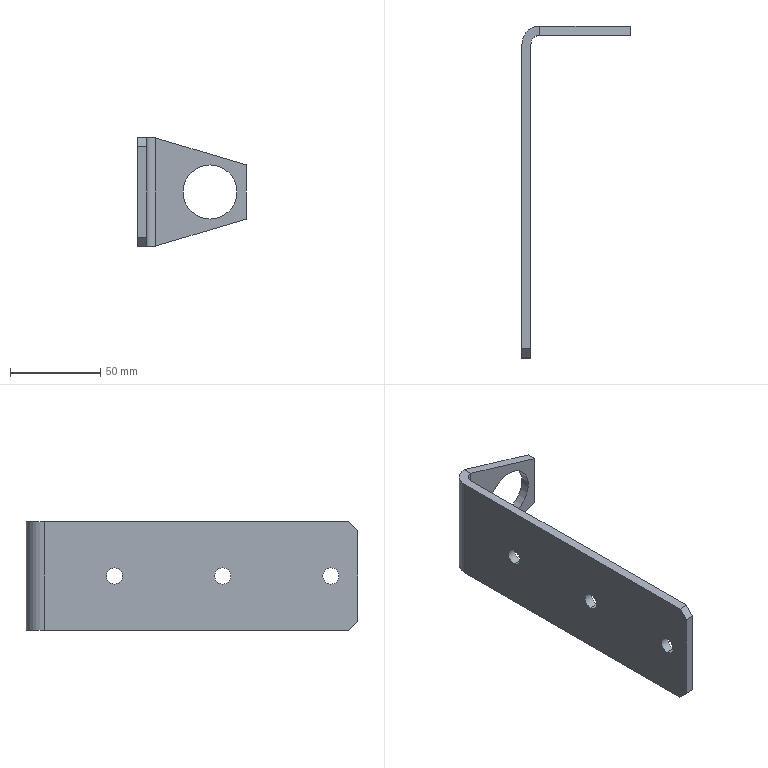Part | SolidWorks | features ICE 3, Chamfer 1, Extrusion 1 | 1 solid | 22 faces | box 60 x 184 x 60 mm | volume 62371 mm3 | plane 12 | cylinder 10 | commonest cylinder face diameters 9 x6 30 x2 10 x1 20 x1
STEP:
#1=CARTESIAN_POINT('',(0.,15.,34.5));
#2=VERTEX_POINT('',#1);
#3=CARTESIAN_POINT('',(0.,15.,25.5));
#4=VERTEX_POINT('',#3);
#5=CARTESIAN_POINT('',(0.,15.,30.));
#6=DIRECTION('',(1.,0.,0.));
#7=DIRECTION('',(0.,0.,-1.));
#8=AXIS2_PLACEMENT_3D('',#5,#6,#7);
#9=CIRCLE('',#8,4.5);
#10=EDGE_CURVE('',#2,#4,#9,.T.);
#11=ORIENTED_EDGE('',*,*,#10,.F.);
#12=CARTESIAN_POINT('',(5.,15.,34.5));
#13=VERTEX_POINT('',#12);
#14=CARTESIAN_POINT('',(-5.,15.,34.5));
#15=DIRECTION('',(1.,0.,0.));
#16=VECTOR('',#15,1000.);
#17=LINE('',#14,#16);
#18=EDGE_CURVE('',#2,#13,#17,.T.);
#19=ORIENTED_EDGE('',*,*,#18,.T.);
#20=CARTESIAN_POINT('',(5.,15.,25.5));
#21=VERTEX_POINT('',#20);
#22=CARTESIAN_POINT('',(5.,15.,30.));
#23=DIRECTION('',(1.,0.,0.));
#24=DIRECTION('',(0.,0.,-1.));
#25=AXIS2_PLACEMENT_3D('',#22,#23,#24);
#26=CIRCLE('',#25,4.5);
#27=EDGE_CURVE('',#13,#21,#26,.T.);
#28=ORIENTED_EDGE('',*,*,#27,.T.);
#29=CARTESIAN_POINT('',(-5.,15.,25.5));
#30=DIRECTION('',(1.,0.,0.));
#31=VECTOR('',#30,1000.);
#32=LINE('',#29,#31);
#33=EDGE_CURVE('',#4,#21,#32,.T.);
#34=ORIENTED_EDGE('',*,*,#33,.F.);
#35=EDGE_LOOP('',(#11,#19,#28,#34));
#36=FACE_OUTER_BOUND('',#35,.T.);
#37=CARTESIAN_POINT('',(-5.,15.,30.));
#38=DIRECTION('',(1.,0.,0.));
#39=DIRECTION('',(0.,0.,-1.));
#40=AXIS2_PLACEMENT_3D('',#37,#38,#39);
#41=CYLINDRICAL_SURFACE('',#40,4.5);
#42=ADVANCED_FACE('',(#36),#41,.F.);
#43=CARTESIAN_POINT('',(0.,75.,34.5));
#44=VERTEX_POINT('',#43);
#45=CARTESIAN_POINT('',(0.,75.,25.5));
#46=VERTEX_POINT('',#45);
#47=CARTESIAN_POINT('',(0.,75.,30.));
#48=DIRECTION('',(1.,0.,0.));
#49=DIRECTION('',(0.,0.,-1.));
#50=AXIS2_PLACEMENT_3D('',#47,#48,#49);
#51=CIRCLE('',#50,4.5);
#52=EDGE_CURVE('',#44,#46,#51,.T.);
#53=ORIENTED_EDGE('',*,*,#52,.F.);
#54=CARTESIAN_POINT('',(5.,75.,34.5));
#55=VERTEX_POINT('',#54);
#56=CARTESIAN_POINT('',(-5.,75.,34.5));
#57=DIRECTION('',(1.,0.,0.));
#58=VECTOR('',#57,1000.);
#59=LINE('',#56,#58);
#60=EDGE_CURVE('',#44,#55,#59,.T.);
#61=ORIENTED_EDGE('',*,*,#60,.T.);
#62=CARTESIAN_POINT('',(5.,75.,25.5));
#63=VERTEX_POINT('',#62);
#64=CARTESIAN_POINT('',(5.,75.,30.));
#65=DIRECTION('',(1.,0.,0.));
#66=DIRECTION('',(0.,0.,-1.));
#67=AXIS2_PLACEMENT_3D('',#64,#65,#66);
#68=CIRCLE('',#67,4.5);
#69=EDGE_CURVE('',#55,#63,#68,.T.);
#70=ORIENTED_EDGE('',*,*,#69,.T.);
#71=CARTESIAN_POINT('',(-5.,75.,25.5));
#72=DIRECTION('',(1.,0.,0.));
#73=VECTOR('',#72,1000.);
#74=LINE('',#71,#73);
#75=EDGE_CURVE('',#46,#63,#74,.T.);
#76=ORIENTED_EDGE('',*,*,#75,.F.);
#77=EDGE_LOOP('',(#53,#61,#70,#76));
#78=FACE_OUTER_BOUND('',#77,.T.);
#79=CARTESIAN_POINT('',(-5.,75.,30.));
#80=DIRECTION('',(1.,0.,0.));
#81=DIRECTION('',(0.,0.,-1.));
#82=AXIS2_PLACEMENT_3D('',#79,#80,#81);
#83=CYLINDRICAL_SURFACE('',#82,4.5);
#84=ADVANCED_FACE('',(#78),#83,.F.);
#85=CARTESIAN_POINT('',(0.,135.,34.5));
#86=VERTEX_POINT('',#85);
#87=CARTESIAN_POINT('',(0.,135.,25.5));
#88=VERTEX_POINT('',#87);
#89=CARTESIAN_POINT('',(0.,135.,30.));
#90=DIRECTION('',(1.,0.,0.));
#91=DIRECTION('',(0.,0.,-1.));
#92=AXIS2_PLACEMENT_3D('',#89,#90,#91);
#93=CIRCLE('',#92,4.5);
#94=EDGE_CURVE('',#86,#88,#93,.T.);
#95=ORIENTED_EDGE('',*,*,#94,.F.);
#96=CARTESIAN_POINT('',(5.,135.,34.5));
#97=VERTEX_POINT('',#96);
#98=CARTESIAN_POINT('',(-5.,135.,34.5));
#99=DIRECTION('',(1.,0.,0.));
#100=VECTOR('',#99,1000.);
#101=LINE('',#98,#100);
#102=EDGE_CURVE('',#86,#97,#101,.T.);
#103=ORIENTED_EDGE('',*,*,#102,.T.);
#104=CARTESIAN_POINT('',(5.,135.,25.5));
#105=VERTEX_POINT('',#104);
#106=CARTESIAN_POINT('',(5.,135.,30.));
#107=DIRECTION('',(1.,0.,0.));
#108=DIRECTION('',(0.,0.,-1.));
#109=AXIS2_PLACEMENT_3D('',#106,#107,#108);
#110=CIRCLE('',#109,4.5);
#111=EDGE_CURVE('',#97,#105,#110,.T.);
#112=ORIENTED_EDGE('',*,*,#111,.T.);
#113=CARTESIAN_POINT('',(-5.,135.,25.5));
#114=DIRECTION('',(1.,0.,0.));
#115=VECTOR('',#114,1000.);
#116=LINE('',#113,#115);
#117=EDGE_CURVE('',#88,#105,#116,.T.);
#118=ORIENTED_EDGE('',*,*,#117,.F.);
#119=EDGE_LOOP('',(#95,#103,#112,#118));
#120=FACE_OUTER_BOUND('',#119,.T.);
#121=CARTESIAN_POINT('',(-5.,135.,30.));
#122=DIRECTION('',(1.,0.,0.));
#123=DIRECTION('',(0.,0.,-1.));
#124=AXIS2_PLACEMENT_3D('',#121,#122,#123);
#125=CYLINDRICAL_SURFACE('',#124,4.5);
#126=ADVANCED_FACE('',(#120),#125,.F.);
#127=CARTESIAN_POINT('',(40.,179.,15.));
#128=VERTEX_POINT('',#127);
#129=CARTESIAN_POINT('',(40.,179.,45.));
#130=VERTEX_POINT('',#129);
#131=CARTESIAN_POINT('',(40.,179.,30.));
#132=DIRECTION('',(0.,1.,0.));
#133=DIRECTION('',(0.,0.,1.));
#134=AXIS2_PLACEMENT_3D('',#131,#132,#133);
#135=CIRCLE('',#134,15.);
#136=EDGE_CURVE('',#128,#130,#135,.T.);
#137=ORIENTED_EDGE('',*,*,#136,.F.);
#138=CARTESIAN_POINT('',(40.,184.,15.));
#139=VERTEX_POINT('',#138);
#140=CARTESIAN_POINT('',(40.,124.,15.));
#141=DIRECTION('',(0.,1.,0.));
#142=VECTOR('',#141,1000.);
#143=LINE('',#140,#142);
#144=EDGE_CURVE('',#128,#139,#143,.T.);
#145=ORIENTED_EDGE('',*,*,#144,.T.);
#146=CARTESIAN_POINT('',(40.,184.,45.));
#147=VERTEX_POINT('',#146);
#148=CARTESIAN_POINT('',(40.,184.,30.));
#149=DIRECTION('',(0.,1.,0.));
#150=DIRECTION('',(0.,0.,1.));
#151=AXIS2_PLACEMENT_3D('',#148,#149,#150);
#152=CIRCLE('',#151,15.);
#153=EDGE_CURVE('',#139,#147,#152,.T.);
#154=ORIENTED_EDGE('',*,*,#153,.T.);
#155=CARTESIAN_POINT('',(40.,124.,45.));
#156=DIRECTION('',(0.,1.,0.));
#157=VECTOR('',#156,1000.);
#158=LINE('',#155,#157);
#159=EDGE_CURVE('',#130,#147,#158,.T.);
#160=ORIENTED_EDGE('',*,*,#159,.F.);
#161=EDGE_LOOP('',(#137,#145,#154,#160));
#162=FACE_OUTER_BOUND('',#161,.T.);
#163=CARTESIAN_POINT('',(40.,124.,30.));
#164=DIRECTION('',(0.,1.,0.));
#165=DIRECTION('',(0.,0.,1.));
#166=AXIS2_PLACEMENT_3D('',#163,#164,#165);
#167=CYLINDRICAL_SURFACE('',#166,15.);
#168=ADVANCED_FACE('',(#162),#167,.F.);
#169=CARTESIAN_POINT('',(0.,0.,55.));
#170=VERTEX_POINT('',#169);
#171=CARTESIAN_POINT('',(0.,0.,5.));
#172=VERTEX_POINT('',#171);
#173=CARTESIAN_POINT('',(0.,0.,60.));
#174=DIRECTION('',(0.,0.,-1.));
#175=VECTOR('',#174,1000.);
#176=LINE('',#173,#175);
#177=EDGE_CURVE('',#170,#172,#176,.T.);
#178=ORIENTED_EDGE('',*,*,#177,.T.);
#179=CARTESIAN_POINT('',(5.,0.,5.));
#180=VERTEX_POINT('',#179);
#181=CARTESIAN_POINT('',(5.,0.,5.));
#182=DIRECTION('',(1.,0.,0.));
#183=VECTOR('',#182,1000.);
#184=LINE('',#181,#183);
#185=EDGE_CURVE('',#172,#180,#184,.T.);
#186=ORIENTED_EDGE('',*,*,#185,.T.);
#187=CARTESIAN_POINT('',(5.,0.,55.));
#188=VERTEX_POINT('',#187);
#189=CARTESIAN_POINT('',(5.,0.,60.));
#190=DIRECTION('',(0.,0.,-1.));
#191=VECTOR('',#190,1000.);
#192=LINE('',#189,#191);
#193=EDGE_CURVE('',#188,#180,#192,.T.);
#194=ORIENTED_EDGE('',*,*,#193,.F.);
#195=CARTESIAN_POINT('',(0.,0.,55.));
#196=DIRECTION('',(-1.,0.,0.));
#197=VECTOR('',#196,1000.);
#198=LINE('',#195,#197);
#199=EDGE_CURVE('',#188,#170,#198,.T.);
#200=ORIENTED_EDGE('',*,*,#199,.T.);
#201=EDGE_LOOP('',(#178,#186,#194,#200));
#202=FACE_OUTER_BOUND('',#201,.T.);
#203=CARTESIAN_POINT('',(0.,0.,60.));
#204=DIRECTION('',(0.,1.,0.));
#205=DIRECTION('',(0.,0.,1.));
#206=AXIS2_PLACEMENT_3D('',#203,#204,#205);
#207=PLANE('',#206);
#208=ADVANCED_FACE('',(#202),#207,.F.);
#209=CARTESIAN_POINT('',(5.,15.,30.));
#210=DIRECTION('',(1.,0.,0.));
#211=DIRECTION('',(0.,0.,-1.));
#212=AXIS2_PLACEMENT_3D('',#209,#210,#211);
#213=CIRCLE('',#212,4.5);
#214=EDGE_CURVE('',#21,#13,#213,.T.);
#215=ORIENTED_EDGE('',*,*,#214,.F.);
#216=ORIENTED_EDGE('',*,*,#27,.F.);
#217=EDGE_LOOP('',(#215,#216));
#218=FACE_BOUND('',#217,.T.);
#219=CARTESIAN_POINT('',(5.,75.,30.));
#220=DIRECTION('',(1.,0.,0.));
#221=DIRECTION('',(0.,0.,-1.));
#222=AXIS2_PLACEMENT_3D('',#219,#220,#221);
#223=CIRCLE('',#222,4.5);
#224=EDGE_CURVE('',#63,#55,#223,.T.);
#225=ORIENTED_EDGE('',*,*,#224,.F.);
#226=ORIENTED_EDGE('',*,*,#69,.F.);
#227=EDGE_LOOP('',(#225,#226));
#228=FACE_BOUND('',#227,.T.);
#229=CARTESIAN_POINT('',(5.,135.,30.));
#230=DIRECTION('',(1.,0.,0.));
#231=DIRECTION('',(0.,0.,-1.));
#232=AXIS2_PLACEMENT_3D('',#229,#230,#231);
#233=CIRCLE('',#232,4.5);
#234=EDGE_CURVE('',#105,#97,#233,.T.);
#235=ORIENTED_EDGE('',*,*,#234,.F.);
#236=ORIENTED_EDGE('',*,*,#111,.F.);
#237=EDGE_LOOP('',(#235,#236));
#238=FACE_BOUND('',#237,.T.);
#239=ORIENTED_EDGE('',*,*,#193,.T.);
#240=CARTESIAN_POINT('',(5.,5.,0.));
#241=VERTEX_POINT('',#240);
#242=CARTESIAN_POINT('',(5.,0.,5.));
#243=DIRECTION('',(0.,0.7071,-0.7071));
#244=VECTOR('',#243,1000.);
#245=LINE('',#242,#244);
#246=EDGE_CURVE('',#180,#241,#245,.T.);
#247=ORIENTED_EDGE('',*,*,#246,.T.);
#248=CARTESIAN_POINT('',(5.,174.,0.));
#249=VERTEX_POINT('',#248);
#250=CARTESIAN_POINT('',(5.,0.,0.));
#251=DIRECTION('',(0.,1.,0.));
#252=VECTOR('',#251,1000.);
#253=LINE('',#250,#252);
#254=EDGE_CURVE('',#241,#249,#253,.T.);
#255=ORIENTED_EDGE('',*,*,#254,.T.);
#256=CARTESIAN_POINT('',(5.,174.,60.));
#257=VERTEX_POINT('',#256);
#258=CARTESIAN_POINT('',(5.,174.,60.));
#259=DIRECTION('',(0.,0.,-1.));
#260=VECTOR('',#259,1000.);
#261=LINE('',#258,#260);
#262=EDGE_CURVE('',#257,#249,#261,.T.);
#263=ORIENTED_EDGE('',*,*,#262,.F.);
#264=CARTESIAN_POINT('',(5.,5.,60.));
#265=VERTEX_POINT('',#264);
#266=CARTESIAN_POINT('',(5.,0.,60.));
#267=DIRECTION('',(0.,1.,0.));
#268=VECTOR('',#267,1000.);
#269=LINE('',#266,#268);
#270=EDGE_CURVE('',#265,#257,#269,.T.);
#271=ORIENTED_EDGE('',*,*,#270,.F.);
#272=CARTESIAN_POINT('',(5.,5.,60.));
#273=DIRECTION('',(0.,-0.7071,-0.7071));
#274=VECTOR('',#273,1000.);
#275=LINE('',#272,#274);
#276=EDGE_CURVE('',#265,#188,#275,.T.);
#277=ORIENTED_EDGE('',*,*,#276,.T.);
#278=EDGE_LOOP('',(#239,#247,#255,#263,#271,#277));
#279=FACE_OUTER_BOUND('',#278,.T.);
#280=CARTESIAN_POINT('',(5.,0.,60.));
#281=DIRECTION('',(-1.,0.,0.));
#282=DIRECTION('',(0.,0.,1.));
#283=AXIS2_PLACEMENT_3D('',#280,#281,#282);
#284=PLANE('',#283);
#285=ADVANCED_FACE('',(#218,#228,#238,#279),#284,.F.);
#286=CARTESIAN_POINT('',(10.,179.,0.));
#287=VERTEX_POINT('',#286);
#288=CARTESIAN_POINT('',(10.,174.,0.));
#289=DIRECTION('',(0.,0.,-1.));
#290=DIRECTION('',(-1.,0.,0.));
#291=AXIS2_PLACEMENT_3D('',#288,#289,#290);
#292=CIRCLE('',#291,5.);
#293=EDGE_CURVE('',#249,#287,#292,.T.);
#294=ORIENTED_EDGE('',*,*,#293,.T.);
#295=CARTESIAN_POINT('',(10.,179.,60.));
#296=VERTEX_POINT('',#295);
#297=CARTESIAN_POINT('',(10.,179.,60.));
#298=DIRECTION('',(0.,0.,-1.));
#299=VECTOR('',#298,1000.);
#300=LINE('',#297,#299);
#301=EDGE_CURVE('',#296,#287,#300,.T.);
#302=ORIENTED_EDGE('',*,*,#301,.F.);
#303=CARTESIAN_POINT('',(10.,174.,60.));
#304=DIRECTION('',(0.,0.,-1.));
#305=DIRECTION('',(-1.,0.,0.));
#306=AXIS2_PLACEMENT_3D('',#303,#304,#305);
#307=CIRCLE('',#306,5.);
#308=EDGE_CURVE('',#257,#296,#307,.T.);
#309=ORIENTED_EDGE('',*,*,#308,.F.);
#310=ORIENTED_EDGE('',*,*,#262,.T.);
#311=EDGE_LOOP('',(#294,#302,#309,#310));
#312=FACE_OUTER_BOUND('',#311,.T.);
#313=CARTESIAN_POINT('',(10.,174.,60.));
#314=DIRECTION('',(0.,0.,-1.));
#315=DIRECTION('',(-1.,0.,0.));
#316=AXIS2_PLACEMENT_3D('',#313,#314,#315);
#317=CYLINDRICAL_SURFACE('',#316,5.);
#318=ADVANCED_FACE('',(#312),#317,.F.);
#319=CARTESIAN_POINT('',(40.,179.,30.));
#320=DIRECTION('',(0.,1.,0.));
#321=DIRECTION('',(0.,0.,1.));
#322=AXIS2_PLACEMENT_3D('',#319,#320,#321);
#323=CIRCLE('',#322,15.);
#324=EDGE_CURVE('',#130,#128,#323,.T.);
#325=ORIENTED_EDGE('',*,*,#324,.T.);
#326=ORIENTED_EDGE('',*,*,#136,.T.);
#327=EDGE_LOOP('',(#325,#326));
#328=FACE_BOUND('',#327,.T.);
#329=ORIENTED_EDGE('',*,*,#301,.T.);
#330=CARTESIAN_POINT('',(60.,179.,15.));
#331=VERTEX_POINT('',#330);
#332=CARTESIAN_POINT('',(26.514,179.,4.954));
#333=DIRECTION('',(0.9578,0.,0.2873));
#334=VECTOR('',#333,1000.);
#335=LINE('',#332,#334);
#336=EDGE_CURVE('',#287,#331,#335,.T.);
#337=ORIENTED_EDGE('',*,*,#336,.T.);
#338=CARTESIAN_POINT('',(60.,179.,45.));
#339=VERTEX_POINT('',#338);
#340=CARTESIAN_POINT('',(60.,179.,60.));
#341=DIRECTION('',(0.,0.,-1.));
#342=VECTOR('',#341,1000.);
#343=LINE('',#340,#342);
#344=EDGE_CURVE('',#339,#331,#343,.T.);
#345=ORIENTED_EDGE('',*,*,#344,.F.);
#346=CARTESIAN_POINT('',(10.,179.,60.));
#347=DIRECTION('',(-0.9578,0.,0.2873));
#348=VECTOR('',#347,1000.);
#349=LINE('',#346,#348);
#350=EDGE_CURVE('',#339,#296,#349,.T.);
#351=ORIENTED_EDGE('',*,*,#350,.T.);
#352=EDGE_LOOP('',(#329,#337,#345,#351));
#353=FACE_OUTER_BOUND('',#352,.T.);
#354=CARTESIAN_POINT('',(10.,179.,60.));
#355=DIRECTION('',(0.,1.,0.));
#356=DIRECTION('',(0.,0.,1.));
#357=AXIS2_PLACEMENT_3D('',#354,#355,#356);
#358=PLANE('',#357);
#359=ADVANCED_FACE('',(#328,#353),#358,.F.);
#360=ORIENTED_EDGE('',*,*,#344,.T.);
#361=CARTESIAN_POINT('',(60.,184.,15.));
#362=VERTEX_POINT('',#361);
#363=CARTESIAN_POINT('',(60.,124.,15.));
#364=DIRECTION('',(0.,1.,0.));
#365=VECTOR('',#364,1000.);
#366=LINE('',#363,#365);
#367=EDGE_CURVE('',#331,#362,#366,.T.);
#368=ORIENTED_EDGE('',*,*,#367,.T.);
#369=CARTESIAN_POINT('',(60.,184.,45.));
#370=VERTEX_POINT('',#369);
#371=CARTESIAN_POINT('',(60.,184.,60.));
#372=DIRECTION('',(0.,0.,-1.));
#373=VECTOR('',#372,1000.);
#374=LINE('',#371,#373);
#375=EDGE_CURVE('',#370,#362,#374,.T.);
#376=ORIENTED_EDGE('',*,*,#375,.F.);
#377=CARTESIAN_POINT('',(60.,124.,45.));
#378=DIRECTION('',(0.,1.,0.));
#379=VECTOR('',#378,1000.);
#380=LINE('',#377,#379);
#381=EDGE_CURVE('',#339,#370,#380,.T.);
#382=ORIENTED_EDGE('',*,*,#381,.F.);
#383=EDGE_LOOP('',(#360,#368,#376,#382));
#384=FACE_OUTER_BOUND('',#383,.T.);
#385=CARTESIAN_POINT('',(60.,184.,60.));
#386=DIRECTION('',(-1.,0.,0.));
#387=DIRECTION('',(0.,0.,1.));
#388=AXIS2_PLACEMENT_3D('',#385,#386,#387);
#389=PLANE('',#388);
#390=ADVANCED_FACE('',(#384),#389,.F.);
#391=CARTESIAN_POINT('',(40.,184.,30.));
#392=DIRECTION('',(0.,1.,0.));
#393=DIRECTION('',(0.,0.,1.));
#394=AXIS2_PLACEMENT_3D('',#391,#392,#393);
#395=CIRCLE('',#394,15.);
#396=EDGE_CURVE('',#147,#139,#395,.T.);
#397=ORIENTED_EDGE('',*,*,#396,.F.);
#398=ORIENTED_EDGE('',*,*,#153,.F.);
#399=EDGE_LOOP('',(#397,#398));
#400=FACE_BOUND('',#399,.T.);
#401=ORIENTED_EDGE('',*,*,#375,.T.);
#402=CARTESIAN_POINT('',(10.,184.,0.));
#403=VERTEX_POINT('',#402);
#404=CARTESIAN_POINT('',(10.,184.,0.));
#405=DIRECTION('',(0.9578,0.,0.2873));
#406=VECTOR('',#405,1000.);
#407=LINE('',#404,#406);
#408=EDGE_CURVE('',#403,#362,#407,.T.);
#409=ORIENTED_EDGE('',*,*,#408,.F.);
#410=CARTESIAN_POINT('',(10.,184.,60.));
#411=VERTEX_POINT('',#410);
#412=CARTESIAN_POINT('',(10.,184.,60.));
#413=DIRECTION('',(0.,0.,-1.));
#414=VECTOR('',#413,1000.);
#415=LINE('',#412,#414);
#416=EDGE_CURVE('',#411,#403,#415,.T.);
#417=ORIENTED_EDGE('',*,*,#416,.F.);
#418=CARTESIAN_POINT('',(60.,184.,45.));
#419=DIRECTION('',(-0.9578,0.,0.2873));
#420=VECTOR('',#419,1000.);
#421=LINE('',#418,#420);
#422=EDGE_CURVE('',#370,#411,#421,.T.);
#423=ORIENTED_EDGE('',*,*,#422,.F.);
#424=EDGE_LOOP('',(#401,#409,#417,#423));
#425=FACE_OUTER_BOUND('',#424,.T.);
#426=CARTESIAN_POINT('',(10.,184.,60.));
#427=DIRECTION('',(0.,-1.,0.));
#428=DIRECTION('',(0.,0.,-1.));
#429=AXIS2_PLACEMENT_3D('',#426,#427,#428);
#430=PLANE('',#429);
#431=ADVANCED_FACE('',(#400,#425),#430,.F.);
#432=CARTESIAN_POINT('',(0.,174.,0.));
#433=VERTEX_POINT('',#432);
#434=CARTESIAN_POINT('',(10.,174.,0.));
#435=DIRECTION('',(0.,0.,1.));
#436=DIRECTION('',(-1.,0.,0.));
#437=AXIS2_PLACEMENT_3D('',#434,#435,#436);
#438=CIRCLE('',#437,10.);
#439=EDGE_CURVE('',#403,#433,#438,.T.);
#440=ORIENTED_EDGE('',*,*,#439,.T.);
#441=CARTESIAN_POINT('',(0.,174.,60.));
#442=VERTEX_POINT('',#441);
#443=CARTESIAN_POINT('',(0.,174.,60.));
#444=DIRECTION('',(0.,0.,-1.));
#445=VECTOR('',#444,1000.);
#446=LINE('',#443,#445);
#447=EDGE_CURVE('',#442,#433,#446,.T.);
#448=ORIENTED_EDGE('',*,*,#447,.F.);
#449=CARTESIAN_POINT('',(10.,174.,60.));
#450=DIRECTION('',(0.,0.,1.));
#451=DIRECTION('',(-1.,0.,0.));
#452=AXIS2_PLACEMENT_3D('',#449,#450,#451);
#453=CIRCLE('',#452,10.);
#454=EDGE_CURVE('',#411,#442,#453,.T.);
#455=ORIENTED_EDGE('',*,*,#454,.F.);
#456=ORIENTED_EDGE('',*,*,#416,.T.);
#457=EDGE_LOOP('',(#440,#448,#455,#456));
#458=FACE_OUTER_BOUND('',#457,.T.);
#459=CARTESIAN_POINT('',(10.,174.,60.));
#460=DIRECTION('',(0.,0.,-1.));
#461=DIRECTION('',(-1.,0.,0.));
#462=AXIS2_PLACEMENT_3D('',#459,#460,#461);
#463=CYLINDRICAL_SURFACE('',#462,10.);
#464=ADVANCED_FACE('',(#458),#463,.T.);
#465=CARTESIAN_POINT('',(0.,15.,30.));
#466=DIRECTION('',(1.,0.,0.));
#467=DIRECTION('',(0.,0.,-1.));
#468=AXIS2_PLACEMENT_3D('',#465,#466,#467);
#469=CIRCLE('',#468,4.5);
#470=EDGE_CURVE('',#4,#2,#469,.T.);
#471=ORIENTED_EDGE('',*,*,#470,.T.);
#472=ORIENTED_EDGE('',*,*,#10,.T.);
#473=EDGE_LOOP('',(#471,#472));
#474=FACE_BOUND('',#473,.T.);
#475=CARTESIAN_POINT('',(0.,75.,30.));
#476=DIRECTION('',(1.,0.,0.));
#477=DIRECTION('',(0.,0.,-1.));
#478=AXIS2_PLACEMENT_3D('',#475,#476,#477);
#479=CIRCLE('',#478,4.5);
#480=EDGE_CURVE('',#46,#44,#479,.T.);
#481=ORIENTED_EDGE('',*,*,#480,.T.);
#482=ORIENTED_EDGE('',*,*,#52,.T.);
#483=EDGE_LOOP('',(#481,#482));
#484=FACE_BOUND('',#483,.T.);
#485=CARTESIAN_POINT('',(0.,135.,30.));
#486=DIRECTION('',(1.,0.,0.));
#487=DIRECTION('',(0.,0.,-1.));
#488=AXIS2_PLACEMENT_3D('',#485,#486,#487);
#489=CIRCLE('',#488,4.5);
#490=EDGE_CURVE('',#88,#86,#489,.T.);
#491=ORIENTED_EDGE('',*,*,#490,.T.);
#492=ORIENTED_EDGE('',*,*,#94,.T.);
#493=EDGE_LOOP('',(#491,#492));
#494=FACE_BOUND('',#493,.T.);
#495=CARTESIAN_POINT('',(0.,5.,0.));
#496=VERTEX_POINT('',#495);
#497=CARTESIAN_POINT('',(0.,0.,0.));
#498=DIRECTION('',(0.,-1.,0.));
#499=VECTOR('',#498,1000.);
#500=LINE('',#497,#499);
#501=EDGE_CURVE('',#433,#496,#500,.T.);
#502=ORIENTED_EDGE('',*,*,#501,.T.);
#503=CARTESIAN_POINT('',(0.,0.,5.));
#504=DIRECTION('',(0.,-0.7071,0.7071));
#505=VECTOR('',#504,1000.);
#506=LINE('',#503,#505);
#507=EDGE_CURVE('',#496,#172,#506,.T.);
#508=ORIENTED_EDGE('',*,*,#507,.T.);
#509=ORIENTED_EDGE('',*,*,#177,.F.);
#510=CARTESIAN_POINT('',(0.,5.,60.));
#511=VERTEX_POINT('',#510);
#512=CARTESIAN_POINT('',(0.,5.,60.));
#513=DIRECTION('',(0.,0.7071,0.7071));
#514=VECTOR('',#513,1000.);
#515=LINE('',#512,#514);
#516=EDGE_CURVE('',#170,#511,#515,.T.);
#517=ORIENTED_EDGE('',*,*,#516,.T.);
#518=CARTESIAN_POINT('',(0.,0.,60.));
#519=DIRECTION('',(0.,-1.,0.));
#520=VECTOR('',#519,1000.);
#521=LINE('',#518,#520);
#522=EDGE_CURVE('',#442,#511,#521,.T.);
#523=ORIENTED_EDGE('',*,*,#522,.F.);
#524=ORIENTED_EDGE('',*,*,#447,.T.);
#525=EDGE_LOOP('',(#502,#508,#509,#517,#523,#524));
#526=FACE_OUTER_BOUND('',#525,.T.);
#527=CARTESIAN_POINT('',(0.,0.,60.));
#528=DIRECTION('',(1.,0.,0.));
#529=DIRECTION('',(0.,0.,-1.));
#530=AXIS2_PLACEMENT_3D('',#527,#528,#529);
#531=PLANE('',#530);
#532=ADVANCED_FACE('',(#474,#484,#494,#526),#531,.F.);
#533=ORIENTED_EDGE('',*,*,#308,.T.);
#534=CARTESIAN_POINT('',(10.,174.,60.));
#535=DIRECTION('',(0.,1.,0.));
#536=VECTOR('',#535,1000.);
#537=LINE('',#534,#536);
#538=EDGE_CURVE('',#296,#411,#537,.T.);
#539=ORIENTED_EDGE('',*,*,#538,.T.);
#540=ORIENTED_EDGE('',*,*,#454,.T.);
#541=ORIENTED_EDGE('',*,*,#522,.T.);
#542=CARTESIAN_POINT('',(10.,5.,60.));
#543=DIRECTION('',(1.,0.,0.));
#544=VECTOR('',#543,1000.);
#545=LINE('',#542,#544);
#546=EDGE_CURVE('',#511,#265,#545,.T.);
#547=ORIENTED_EDGE('',*,*,#546,.T.);
#548=ORIENTED_EDGE('',*,*,#270,.T.);
#549=EDGE_LOOP('',(#533,#539,#540,#541,#547,#548));
#550=FACE_OUTER_BOUND('',#549,.T.);
#551=CARTESIAN_POINT('',(10.,174.,60.));
#552=DIRECTION('',(0.,0.,-1.));
#553=DIRECTION('',(-1.,0.,0.));
#554=AXIS2_PLACEMENT_3D('',#551,#552,#553);
#555=PLANE('',#554);
#556=ADVANCED_FACE('',(#550),#555,.F.);
#557=CARTESIAN_POINT('',(10.,174.,0.));
#558=DIRECTION('',(0.,1.,0.));
#559=VECTOR('',#558,1000.);
#560=LINE('',#557,#559);
#561=EDGE_CURVE('',#287,#403,#560,.T.);
#562=ORIENTED_EDGE('',*,*,#561,.F.);
#563=ORIENTED_EDGE('',*,*,#293,.F.);
#564=ORIENTED_EDGE('',*,*,#254,.F.);
#565=CARTESIAN_POINT('',(0.,5.,0.));
#566=DIRECTION('',(-1.,0.,0.));
#567=VECTOR('',#566,1000.);
#568=LINE('',#565,#567);
#569=EDGE_CURVE('',#241,#496,#568,.T.);
#570=ORIENTED_EDGE('',*,*,#569,.T.);
#571=ORIENTED_EDGE('',*,*,#501,.F.);
#572=ORIENTED_EDGE('',*,*,#439,.F.);
#573=EDGE_LOOP('',(#562,#563,#564,#570,#571,#572));
#574=FACE_OUTER_BOUND('',#573,.T.);
#575=CARTESIAN_POINT('',(10.,174.,0.));
#576=DIRECTION('',(0.,0.,-1.));
#577=DIRECTION('',(-1.,0.,0.));
#578=AXIS2_PLACEMENT_3D('',#575,#576,#577);
#579=PLANE('',#578);
#580=ADVANCED_FACE('',(#574),#579,.T.);
#581=ORIENTED_EDGE('',*,*,#507,.F.);
#582=ORIENTED_EDGE('',*,*,#569,.F.);
#583=ORIENTED_EDGE('',*,*,#246,.F.);
#584=ORIENTED_EDGE('',*,*,#185,.F.);
#585=EDGE_LOOP('',(#581,#582,#583,#584));
#586=FACE_OUTER_BOUND('',#585,.T.);
#587=CARTESIAN_POINT('',(0.,0.,5.));
#588=DIRECTION('',(0.,-0.7071,-0.7071));
#589=DIRECTION('',(-1.,0.,0.));
#590=AXIS2_PLACEMENT_3D('',#587,#588,#589);
#591=PLANE('',#590);
#592=ADVANCED_FACE('',(#586),#591,.T.);
#593=ORIENTED_EDGE('',*,*,#516,.F.);
#594=ORIENTED_EDGE('',*,*,#199,.F.);
#595=ORIENTED_EDGE('',*,*,#276,.F.);
#596=ORIENTED_EDGE('',*,*,#546,.F.);
#597=EDGE_LOOP('',(#593,#594,#595,#596));
#598=FACE_OUTER_BOUND('',#597,.T.);
#599=CARTESIAN_POINT('',(10.,5.,60.));
#600=DIRECTION('',(0.,0.7071,-0.7071));
#601=DIRECTION('',(1.,0.,0.));
#602=AXIS2_PLACEMENT_3D('',#599,#600,#601);
#603=PLANE('',#602);
#604=ADVANCED_FACE('',(#598),#603,.F.);
#605=ORIENTED_EDGE('',*,*,#144,.F.);
#606=ORIENTED_EDGE('',*,*,#324,.F.);
#607=ORIENTED_EDGE('',*,*,#159,.T.);
#608=ORIENTED_EDGE('',*,*,#396,.T.);
#609=EDGE_LOOP('',(#605,#606,#607,#608));
#610=FACE_OUTER_BOUND('',#609,.T.);
#611=CARTESIAN_POINT('',(40.,124.,30.));
#612=DIRECTION('',(0.,1.,0.));
#613=DIRECTION('',(0.,0.,1.));
#614=AXIS2_PLACEMENT_3D('',#611,#612,#613);
#615=CYLINDRICAL_SURFACE('',#614,15.);
#616=ADVANCED_FACE('',(#610),#615,.F.);
#617=ORIENTED_EDGE('',*,*,#561,.T.);
#618=ORIENTED_EDGE('',*,*,#408,.T.);
#619=ORIENTED_EDGE('',*,*,#367,.F.);
#620=ORIENTED_EDGE('',*,*,#336,.F.);
#621=EDGE_LOOP('',(#617,#618,#619,#620));
#622=FACE_OUTER_BOUND('',#621,.T.);
#623=CARTESIAN_POINT('',(10.,124.,0.));
#624=DIRECTION('',(-0.2873,0.,0.9578));
#625=DIRECTION('',(0.9578,0.,0.2873));
#626=AXIS2_PLACEMENT_3D('',#623,#624,#625);
#627=PLANE('',#626);
#628=ADVANCED_FACE('',(#622),#627,.F.);
#629=ORIENTED_EDGE('',*,*,#381,.T.);
#630=ORIENTED_EDGE('',*,*,#422,.T.);
#631=ORIENTED_EDGE('',*,*,#538,.F.);
#632=ORIENTED_EDGE('',*,*,#350,.F.);
#633=EDGE_LOOP('',(#629,#630,#631,#632));
#634=FACE_OUTER_BOUND('',#633,.T.);
#635=CARTESIAN_POINT('',(60.,124.,45.));
#636=DIRECTION('',(-0.2873,0.,-0.9578));
#637=DIRECTION('',(-0.9578,0.,0.2873));
#638=AXIS2_PLACEMENT_3D('',#635,#636,#637);
#639=PLANE('',#638);
#640=ADVANCED_FACE('',(#634),#639,.F.);
#641=ORIENTED_EDGE('',*,*,#102,.F.);
#642=ORIENTED_EDGE('',*,*,#490,.F.);
#643=ORIENTED_EDGE('',*,*,#117,.T.);
#644=ORIENTED_EDGE('',*,*,#234,.T.);
#645=EDGE_LOOP('',(#641,#642,#643,#644));
#646=FACE_OUTER_BOUND('',#645,.T.);
#647=CARTESIAN_POINT('',(-5.,135.,30.));
#648=DIRECTION('',(1.,0.,0.));
#649=DIRECTION('',(0.,0.,-1.));
#650=AXIS2_PLACEMENT_3D('',#647,#648,#649);
#651=CYLINDRICAL_SURFACE('',#650,4.5);
#652=ADVANCED_FACE('',(#646),#651,.F.);
#653=ORIENTED_EDGE('',*,*,#60,.F.);
#654=ORIENTED_EDGE('',*,*,#480,.F.);
#655=ORIENTED_EDGE('',*,*,#75,.T.);
#656=ORIENTED_EDGE('',*,*,#224,.T.);
#657=EDGE_LOOP('',(#653,#654,#655,#656));
#658=FACE_OUTER_BOUND('',#657,.T.);
#659=CARTESIAN_POINT('',(-5.,75.,30.));
#660=DIRECTION('',(1.,0.,0.));
#661=DIRECTION('',(0.,0.,-1.));
#662=AXIS2_PLACEMENT_3D('',#659,#660,#661);
#663=CYLINDRICAL_SURFACE('',#662,4.5);
#664=ADVANCED_FACE('',(#658),#663,.F.);
#665=ORIENTED_EDGE('',*,*,#18,.F.);
#666=ORIENTED_EDGE('',*,*,#470,.F.);
#667=ORIENTED_EDGE('',*,*,#33,.T.);
#668=ORIENTED_EDGE('',*,*,#214,.T.);
#669=EDGE_LOOP('',(#665,#666,#667,#668));
#670=FACE_OUTER_BOUND('',#669,.T.);
#671=CARTESIAN_POINT('',(-5.,15.,30.));
#672=DIRECTION('',(1.,0.,0.));
#673=DIRECTION('',(0.,0.,-1.));
#674=AXIS2_PLACEMENT_3D('',#671,#672,#673);
#675=CYLINDRICAL_SURFACE('',#674,4.5);
#676=ADVANCED_FACE('',(#670),#675,.F.);
#677=CLOSED_SHELL('',(#42,#84,#126,#168,#208,#285,#318,#359,#390,#431,#464,#532,#556,#580,#592,#604,#616,#628,#640,#652,#664,#676));
#678=MANIFOLD_SOLID_BREP('',#677);
#679=CARTESIAN_POINT('',(0.,0.,0.));
#680=DIRECTION('',(0.,0.,1.));
#681=DIRECTION('',(1.,0.,0.));
#682=AXIS2_PLACEMENT_3D('',#679,#680,#681);
#683=(LENGTH_UNIT()NAMED_UNIT(*)SI_UNIT(.MILLI.,.METRE.));
#684=UNCERTAINTY_MEASURE_WITH_UNIT(LENGTH_MEASURE(0.00001),#683,'','');
#685=(NAMED_UNIT(*)PLANE_ANGLE_UNIT()SI_UNIT($,.RADIAN.));
#686=(NAMED_UNIT(*)SI_UNIT($,.STERADIAN.)SOLID_ANGLE_UNIT());
#687=(GEOMETRIC_REPRESENTATION_CONTEXT(3)GLOBAL_UNCERTAINTY_ASSIGNED_CONTEXT((#684))GLOBAL_UNIT_ASSIGNED_CONTEXT((#683,#685,#686))REPRESENTATION_CONTEXT('',''));
#688=ADVANCED_BREP_SHAPE_REPRESENTATION('',(#678,#682),#687);